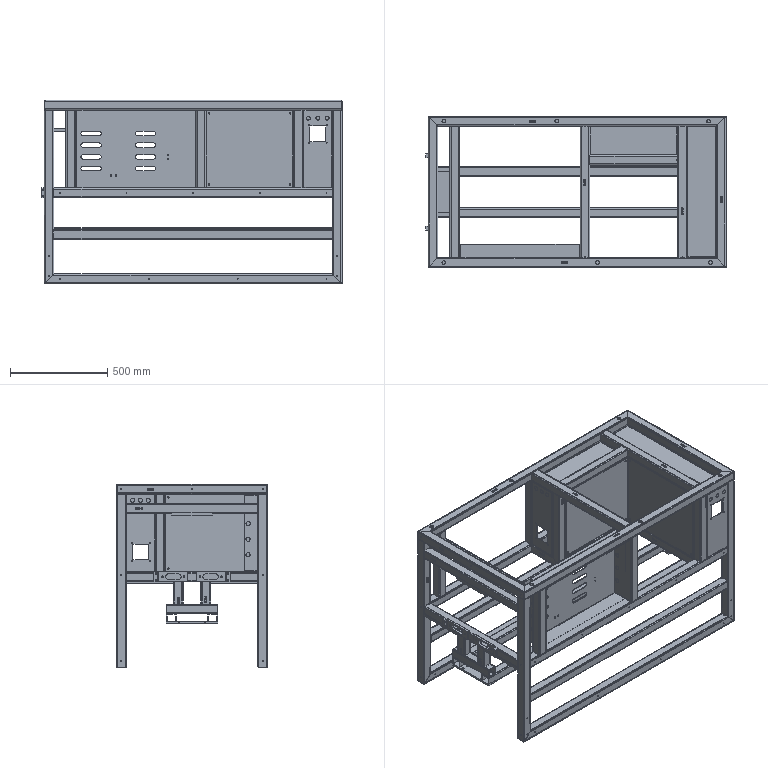Part | SolidWorks | 72 solids | 4836 faces | volume 19240717 mm3 | plane 2681 | spline 1280 | cylinder 857 | cone 18 | commonest cylinder face diameters 6 x182 12 x168 4.2 x96 8 x55 0.4 x36 3.3 x34